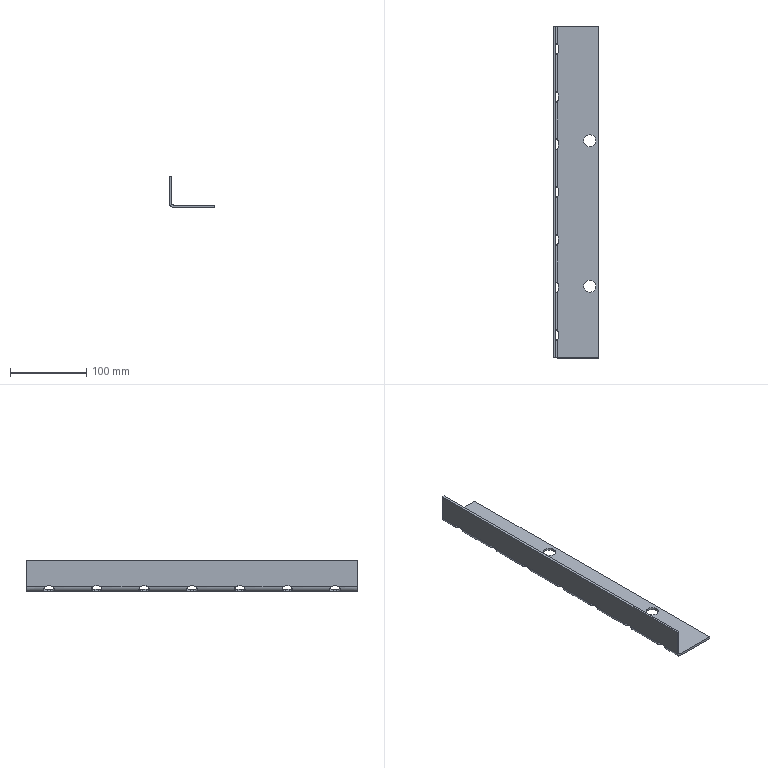Part | NX | features solid 2 | 1 solid | 84 faces | box 60 x 434 x 40 mm | volume 120292 mm3 | cylinder 48 | plane 22 | spline 14 | commonest cylinder face diameters 9 x28 6 x8 12 x8 16 x4